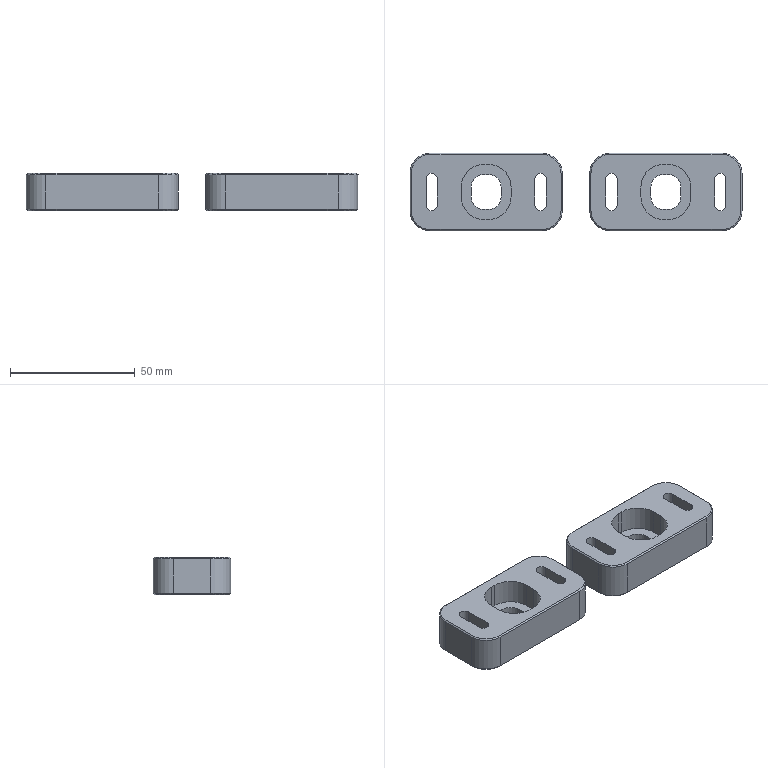Part | 2 solids | 102 faces | box 133 x 31 x 15 mm | volume 42333 mm3 | plane 54 | cylinder 32 | cone 16 | commonest cylinder face diameters 4.5 x8 10 x8 16 x8 18 x8